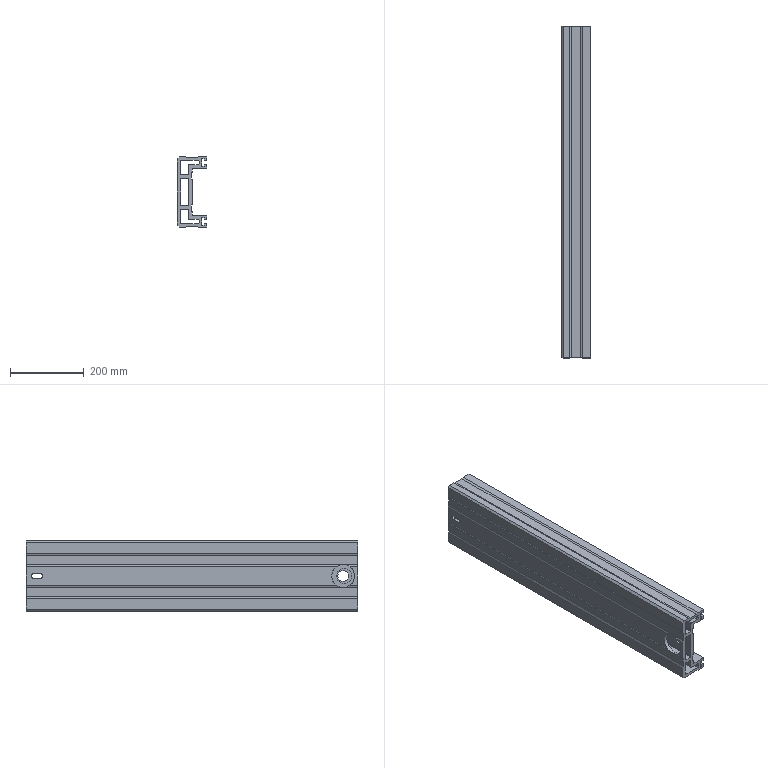Part | STEP file | Main beam | 1 solid | 104 faces | box 80 x 900 x 190 mm | volume 4670487 mm3 | plane 76 | cylinder 28 | commonest cylinder face diameters 4 x18 11.5 x4 30 x2 41 x2 62 x2